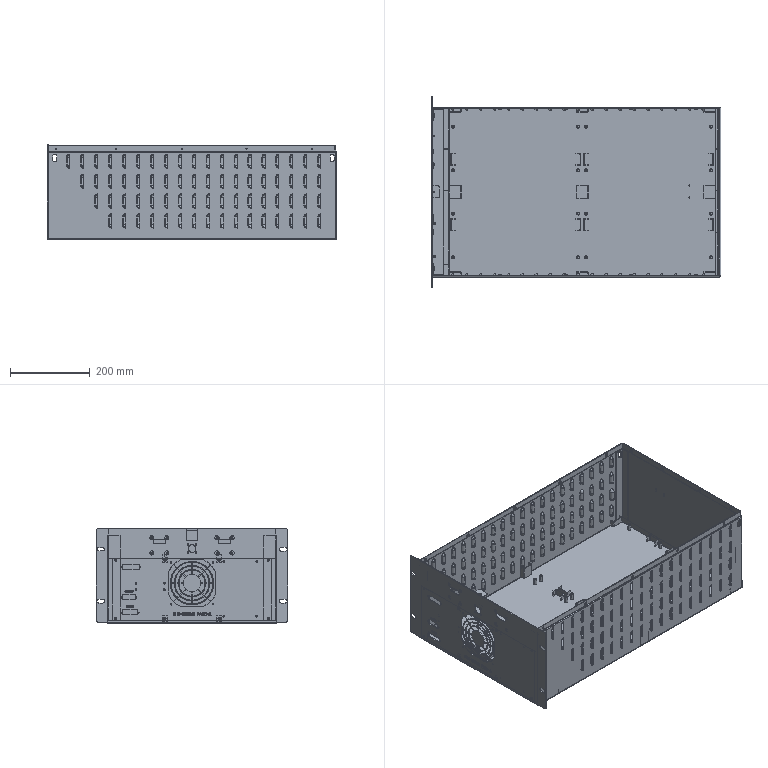Part | NX | features BREP 3 | 3 solids | 3121 faces | volume 1890874 mm3 | plane 1175 | cylinder 854 | sphere 560 | torus 280 | spline 236 | cone 16 | commonest cylinder face diameters 4 x263 12 x140 16 x140 3 x33 1 x32 5 x32